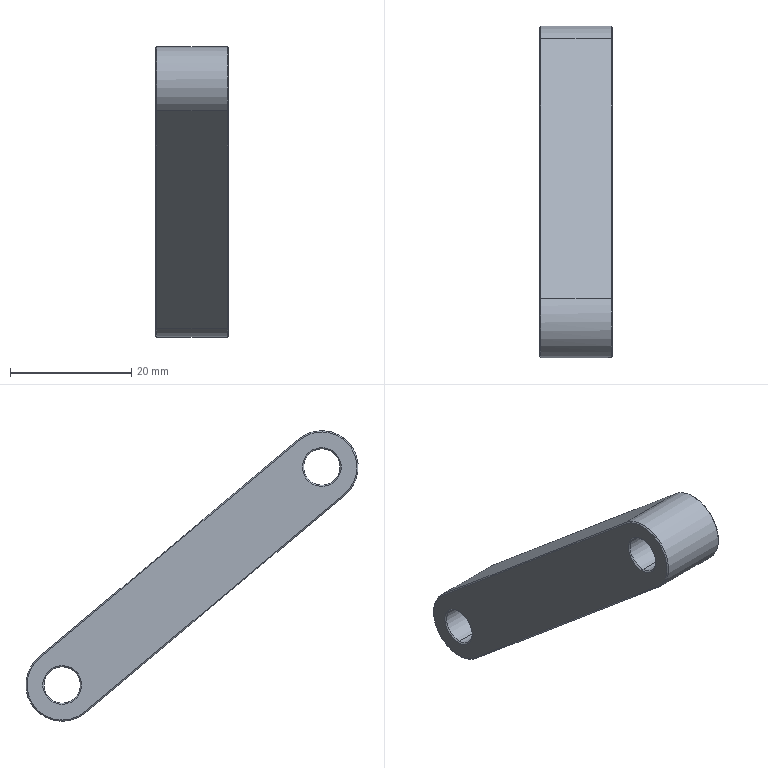Part | STEP file | 2010 | 1 solid | 29 faces | box 12 x 54.895 x 48 mm | volume 8735 mm3 | cone 14 | plane 8 | cylinder 7 | commonest cylinder face diameters 6 x4 12 x3